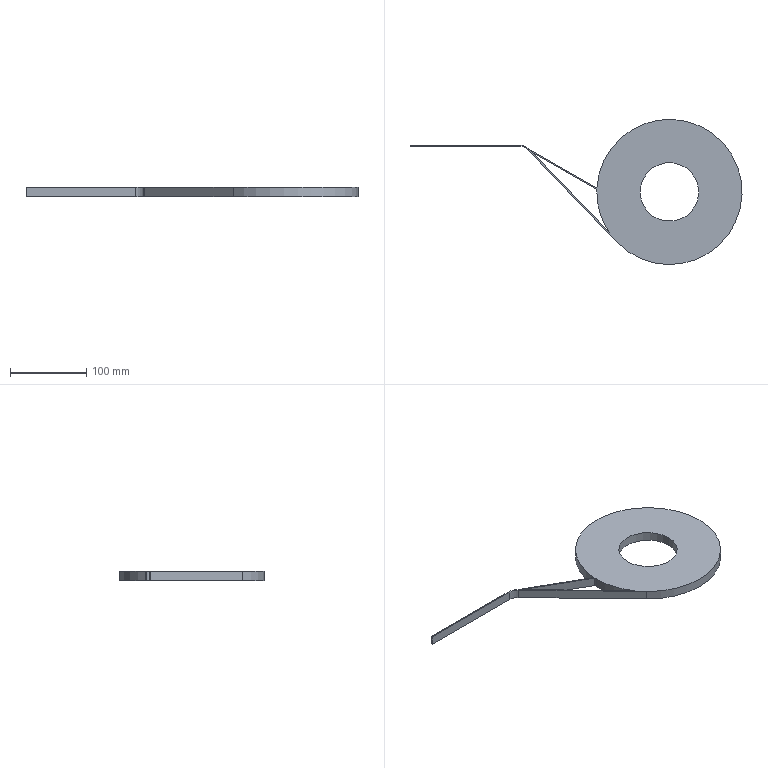Part | STEP file | Mount electronic clip linear-type part | 1 solid | 19 faces | box 434.57 x 190 x 12 mm | volume 291791 mm3 | plane 12 | cylinder 7 | commonest cylinder face diameters 190 x3 76.5 x2 30 x1 32.6 x1
STEP:
#1=CARTESIAN_POINT('',(0.,0.,0.));
#2=DIRECTION('',(0.,0.,1.));
#3=DIRECTION('',(1.,0.,0.));
#4=AXIS2_PLACEMENT_3D('',#1,#2,#3);
#5=CARTESIAN_POINT('',(-95.,0.,6.));
#6=VERTEX_POINT('',#5);
#7=CARTESIAN_POINT('',(-78.379,-53.682,6.));
#8=VERTEX_POINT('',#7);
#9=CARTESIAN_POINT('',(0.,0.,6.));
#10=DIRECTION('',(0.,0.,1.));
#11=DIRECTION('',(1.,0.,0.));
#12=AXIS2_PLACEMENT_3D('',#9,#10,#11);
#13=CIRCLE('',#12,95.);
#14=CARTESIAN_POINT('',(0.,0.,6.));
#15=DIRECTION('',(0.,0.,-1.));
#16=DIRECTION('',(-1.,0.,0.));
#17=AXIS2_PLACEMENT_3D('',#14,#15,#16);
#18=CYLINDRICAL_SURFACE('',#17,95.);
#19=CARTESIAN_POINT('',(9.425,0.));
#20=DIRECTION('',(-1.,0.));
#21=VECTOR('',#20,1.);
#22=LINE('',#19,#21);
#23=(GEOMETRIC_REPRESENTATION_CONTEXT(2)PARAMETRIC_REPRESENTATION_CONTEXT()REPRESENTATION_CONTEXT('',''));
#24=DEFINITIONAL_REPRESENTATION('',(#22),#23);
#25=PCURVE('',#18,#24);
#26=CARTESIAN_POINT('',(0.,0.,6.));
#27=DIRECTION('',(0.,0.,1.));
#28=DIRECTION('',(1.,0.,0.));
#29=AXIS2_PLACEMENT_3D('',#26,#27,#28);
#30=PLANE('',#29);
#31=CARTESIAN_POINT('',(0.,0.));
#32=DIRECTION('',(1.,0.));
#33=AXIS2_PLACEMENT_2D('',#31,#32);
#34=CIRCLE('',#33,95.);
#35=(GEOMETRIC_REPRESENTATION_CONTEXT(2)PARAMETRIC_REPRESENTATION_CONTEXT()REPRESENTATION_CONTEXT('',''));
#36=DEFINITIONAL_REPRESENTATION('',(#34),#35);
#37=PCURVE('',#30,#36);
#38=SURFACE_CURVE('',#13,(#25,#37),.PCURVE_S1.);
#39=EDGE_CURVE('',#6,#8,#38,.T.);
#40=ORIENTED_EDGE('',*,*,#39,.F.);
#41=CARTESIAN_POINT('',(-95.,0.,-6.));
#42=VERTEX_POINT('',#41);
#43=CARTESIAN_POINT('',(-95.,0.,6.));
#44=DIRECTION('',(0.,0.,-1.));
#45=VECTOR('',#44,1.);
#46=LINE('',#43,#45);
#47=CARTESIAN_POINT('',(6.283,0.));
#48=DIRECTION('',(0.,1.));
#49=VECTOR('',#48,1.);
#50=LINE('',#47,#49);
#51=(GEOMETRIC_REPRESENTATION_CONTEXT(2)PARAMETRIC_REPRESENTATION_CONTEXT()REPRESENTATION_CONTEXT('',''));
#52=DEFINITIONAL_REPRESENTATION('',(#50),#51);
#53=PCURVE('',#18,#52);
#54=CARTESIAN_POINT('',(0.,0.,6.));
#55=DIRECTION('',(0.,0.,-1.));
#56=DIRECTION('',(-1.,0.,0.));
#57=AXIS2_PLACEMENT_3D('',#54,#55,#56);
#58=CYLINDRICAL_SURFACE('',#57,95.);
#59=CARTESIAN_POINT('',(0.,0.));
#60=DIRECTION('',(0.,1.));
#61=VECTOR('',#60,1.);
#62=LINE('',#59,#61);
#63=(GEOMETRIC_REPRESENTATION_CONTEXT(2)PARAMETRIC_REPRESENTATION_CONTEXT()REPRESENTATION_CONTEXT('',''));
#64=DEFINITIONAL_REPRESENTATION('',(#62),#63);
#65=PCURVE('',#58,#64);
#66=SURFACE_CURVE('',#46,(#53,#65),.PCURVE_S1.);
#67=EDGE_CURVE('',#6,#42,#66,.T.);
#68=ORIENTED_EDGE('',*,*,#67,.T.);
#69=CARTESIAN_POINT('',(-78.379,-53.682,-6.));
#70=VERTEX_POINT('',#69);
#71=CARTESIAN_POINT('',(0.,0.,-6.));
#72=DIRECTION('',(0.,0.,1.));
#73=DIRECTION('',(1.,0.,0.));
#74=AXIS2_PLACEMENT_3D('',#71,#72,#73);
#75=CIRCLE('',#74,95.);
#76=CARTESIAN_POINT('',(9.425,12.));
#77=DIRECTION('',(-1.,0.));
#78=VECTOR('',#77,1.);
#79=LINE('',#76,#78);
#80=(GEOMETRIC_REPRESENTATION_CONTEXT(2)PARAMETRIC_REPRESENTATION_CONTEXT()REPRESENTATION_CONTEXT('',''));
#81=DEFINITIONAL_REPRESENTATION('',(#79),#80);
#82=PCURVE('',#18,#81);
#83=CARTESIAN_POINT('',(0.,0.,-6.));
#84=DIRECTION('',(0.,0.,1.));
#85=DIRECTION('',(1.,0.,0.));
#86=AXIS2_PLACEMENT_3D('',#83,#84,#85);
#87=PLANE('',#86);
#88=CARTESIAN_POINT('',(0.,0.));
#89=DIRECTION('',(1.,0.));
#90=AXIS2_PLACEMENT_2D('',#88,#89);
#91=CIRCLE('',#90,95.);
#92=(GEOMETRIC_REPRESENTATION_CONTEXT(2)PARAMETRIC_REPRESENTATION_CONTEXT()REPRESENTATION_CONTEXT('',''));
#93=DEFINITIONAL_REPRESENTATION('',(#91),#92);
#94=PCURVE('',#87,#93);
#95=SURFACE_CURVE('',#75,(#82,#94),.PCURVE_S1.);
#96=EDGE_CURVE('',#42,#70,#95,.T.);
#97=ORIENTED_EDGE('',*,*,#96,.T.);
#98=CARTESIAN_POINT('',(-78.379,-53.682,6.));
#99=DIRECTION('',(0.,0.,-1.));
#100=VECTOR('',#99,1.);
#101=LINE('',#98,#100);
#102=CARTESIAN_POINT('',(5.683,0.));
#103=DIRECTION('',(0.,1.));
#104=VECTOR('',#103,1.);
#105=LINE('',#102,#104);
#106=(GEOMETRIC_REPRESENTATION_CONTEXT(2)PARAMETRIC_REPRESENTATION_CONTEXT()REPRESENTATION_CONTEXT('',''));
#107=DEFINITIONAL_REPRESENTATION('',(#105),#106);
#108=PCURVE('',#18,#107);
#109=CARTESIAN_POINT('',(-67.519,-64.968,6.));
#110=DIRECTION('',(-0.7206,-0.6934,0.));
#111=DIRECTION('',(0.6934,-0.7206,0.));
#112=AXIS2_PLACEMENT_3D('',#109,#110,#111);
#113=PLANE('',#112);
#114=CARTESIAN_POINT('',(-15.662,0.));
#115=DIRECTION('',(0.,-1.));
#116=VECTOR('',#115,1.);
#117=LINE('',#114,#116);
#118=(GEOMETRIC_REPRESENTATION_CONTEXT(2)PARAMETRIC_REPRESENTATION_CONTEXT()REPRESENTATION_CONTEXT('',''));
#119=DEFINITIONAL_REPRESENTATION('',(#117),#118);
#120=PCURVE('',#113,#119);
#121=SURFACE_CURVE('',#101,(#108,#120),.PCURVE_S1.);
#122=EDGE_CURVE('',#8,#70,#121,.T.);
#123=ORIENTED_EDGE('',*,*,#122,.F.);
#124=EDGE_LOOP('',(#40,#68,#97,#123));
#125=FACE_BOUND('',#124,.T.);
#126=ADVANCED_FACE('',(#125),#18,.T.);
#127=CARTESIAN_POINT('',(-38.25,0.,6.));
#128=VERTEX_POINT('',#127);
#129=CARTESIAN_POINT('',(-38.25,0.,-6.));
#130=VERTEX_POINT('',#129);
#131=CARTESIAN_POINT('',(-38.25,0.,6.));
#132=DIRECTION('',(0.,0.,-1.));
#133=VECTOR('',#132,1.);
#134=LINE('',#131,#133);
#135=CARTESIAN_POINT('',(0.,0.,6.));
#136=DIRECTION('',(0.,0.,-1.));
#137=DIRECTION('',(-1.,0.,0.));
#138=AXIS2_PLACEMENT_3D('',#135,#136,#137);
#139=CYLINDRICAL_SURFACE('',#138,38.25);
#140=CARTESIAN_POINT('',(6.283,0.));
#141=DIRECTION('',(0.,1.));
#142=VECTOR('',#141,1.);
#143=LINE('',#140,#142);
#144=(GEOMETRIC_REPRESENTATION_CONTEXT(2)PARAMETRIC_REPRESENTATION_CONTEXT()REPRESENTATION_CONTEXT('',''));
#145=DEFINITIONAL_REPRESENTATION('',(#143),#144);
#146=PCURVE('',#139,#145);
#147=CARTESIAN_POINT('',(0.,0.,6.));
#148=DIRECTION('',(0.,0.,-1.));
#149=DIRECTION('',(-1.,0.,0.));
#150=AXIS2_PLACEMENT_3D('',#147,#148,#149);
#151=CYLINDRICAL_SURFACE('',#150,38.25);
#152=CARTESIAN_POINT('',(0.,0.));
#153=DIRECTION('',(0.,1.));
#154=VECTOR('',#153,1.);
#155=LINE('',#152,#154);
#156=(GEOMETRIC_REPRESENTATION_CONTEXT(2)PARAMETRIC_REPRESENTATION_CONTEXT()REPRESENTATION_CONTEXT('',''));
#157=DEFINITIONAL_REPRESENTATION('',(#155),#156);
#158=PCURVE('',#151,#157);
#159=SURFACE_CURVE('',#134,(#146,#158),.PCURVE_S1.);
#160=EDGE_CURVE('',#128,#130,#159,.T.);
#161=ORIENTED_EDGE('',*,*,#160,.T.);
#162=CARTESIAN_POINT('',(38.25,0.,-6.));
#163=VERTEX_POINT('',#162);
#164=CARTESIAN_POINT('',(0.,0.,-6.));
#165=DIRECTION('',(0.,0.,1.));
#166=DIRECTION('',(1.,0.,0.));
#167=AXIS2_PLACEMENT_3D('',#164,#165,#166);
#168=CIRCLE('',#167,38.25);
#169=CARTESIAN_POINT('',(9.425,12.));
#170=DIRECTION('',(-1.,0.));
#171=VECTOR('',#170,1.);
#172=LINE('',#169,#171);
#173=(GEOMETRIC_REPRESENTATION_CONTEXT(2)PARAMETRIC_REPRESENTATION_CONTEXT()REPRESENTATION_CONTEXT('',''));
#174=DEFINITIONAL_REPRESENTATION('',(#172),#173);
#175=PCURVE('',#139,#174);
#176=CARTESIAN_POINT('',(0.,0.));
#177=DIRECTION('',(1.,0.));
#178=AXIS2_PLACEMENT_2D('',#176,#177);
#179=CIRCLE('',#178,38.25);
#180=(GEOMETRIC_REPRESENTATION_CONTEXT(2)PARAMETRIC_REPRESENTATION_CONTEXT()REPRESENTATION_CONTEXT('',''));
#181=DEFINITIONAL_REPRESENTATION('',(#179),#180);
#182=PCURVE('',#87,#181);
#183=SURFACE_CURVE('',#168,(#175,#182),.PCURVE_S1.);
#184=EDGE_CURVE('',#130,#163,#183,.T.);
#185=ORIENTED_EDGE('',*,*,#184,.T.);
#186=CARTESIAN_POINT('',(38.25,0.,6.));
#187=VERTEX_POINT('',#186);
#188=CARTESIAN_POINT('',(38.25,0.,6.));
#189=DIRECTION('',(0.,0.,-1.));
#190=VECTOR('',#189,1.);
#191=LINE('',#188,#190);
#192=CARTESIAN_POINT('',(3.142,0.));
#193=DIRECTION('',(0.,1.));
#194=VECTOR('',#193,1.);
#195=LINE('',#192,#194);
#196=(GEOMETRIC_REPRESENTATION_CONTEXT(2)PARAMETRIC_REPRESENTATION_CONTEXT()REPRESENTATION_CONTEXT('',''));
#197=DEFINITIONAL_REPRESENTATION('',(#195),#196);
#198=PCURVE('',#139,#197);
#199=CARTESIAN_POINT('',(3.142,0.));
#200=DIRECTION('',(0.,1.));
#201=VECTOR('',#200,1.);
#202=LINE('',#199,#201);
#203=(GEOMETRIC_REPRESENTATION_CONTEXT(2)PARAMETRIC_REPRESENTATION_CONTEXT()REPRESENTATION_CONTEXT('',''));
#204=DEFINITIONAL_REPRESENTATION('',(#202),#203);
#205=PCURVE('',#151,#204);
#206=SURFACE_CURVE('',#191,(#198,#205),.PCURVE_S1.);
#207=EDGE_CURVE('',#187,#163,#206,.T.);
#208=ORIENTED_EDGE('',*,*,#207,.F.);
#209=CARTESIAN_POINT('',(0.,0.,6.));
#210=DIRECTION('',(0.,0.,1.));
#211=DIRECTION('',(1.,0.,0.));
#212=AXIS2_PLACEMENT_3D('',#209,#210,#211);
#213=CIRCLE('',#212,38.25);
#214=CARTESIAN_POINT('',(9.425,0.));
#215=DIRECTION('',(-1.,0.));
#216=VECTOR('',#215,1.);
#217=LINE('',#214,#216);
#218=(GEOMETRIC_REPRESENTATION_CONTEXT(2)PARAMETRIC_REPRESENTATION_CONTEXT()REPRESENTATION_CONTEXT('',''));
#219=DEFINITIONAL_REPRESENTATION('',(#217),#218);
#220=PCURVE('',#139,#219);
#221=CARTESIAN_POINT('',(0.,0.));
#222=DIRECTION('',(1.,0.));
#223=AXIS2_PLACEMENT_2D('',#221,#222);
#224=CIRCLE('',#223,38.25);
#225=(GEOMETRIC_REPRESENTATION_CONTEXT(2)PARAMETRIC_REPRESENTATION_CONTEXT()REPRESENTATION_CONTEXT('',''));
#226=DEFINITIONAL_REPRESENTATION('',(#224),#225);
#227=PCURVE('',#30,#226);
#228=SURFACE_CURVE('',#213,(#220,#227),.PCURVE_S1.);
#229=EDGE_CURVE('',#128,#187,#228,.T.);
#230=ORIENTED_EDGE('',*,*,#229,.F.);
#231=EDGE_LOOP('',(#161,#185,#208,#230));
#232=FACE_BOUND('',#231,.F.);
#233=ADVANCED_FACE('',(#232),#139,.F.);
#234=CARTESIAN_POINT('',(-94.855,5.249,6.));
#235=VERTEX_POINT('',#234);
#236=CARTESIAN_POINT('',(-94.855,5.249,-6.));
#237=VERTEX_POINT('',#236);
#238=CARTESIAN_POINT('',(-94.855,5.249,6.));
#239=DIRECTION('',(0.,0.,-1.));
#240=VECTOR('',#239,1.);
#241=LINE('',#238,#240);
#242=CARTESIAN_POINT('',(0.,0.,6.));
#243=DIRECTION('',(0.,0.,-1.));
#244=DIRECTION('',(-1.,0.,0.));
#245=AXIS2_PLACEMENT_3D('',#242,#243,#244);
#246=CYLINDRICAL_SURFACE('',#245,95.);
#247=CARTESIAN_POINT('',(0.05528,0.));
#248=DIRECTION('',(0.,1.));
#249=VECTOR('',#248,1.);
#250=LINE('',#247,#249);
#251=(GEOMETRIC_REPRESENTATION_CONTEXT(2)PARAMETRIC_REPRESENTATION_CONTEXT()REPRESENTATION_CONTEXT('',''));
#252=DEFINITIONAL_REPRESENTATION('',(#250),#251);
#253=PCURVE('',#246,#252);
#254=CARTESIAN_POINT('',(-21.084,-36.901,195.166));
#255=DIRECTION('',(-0.4961,-0.8683,0.));
#256=DIRECTION('',(0.8683,-0.4961,0.));
#257=AXIS2_PLACEMENT_3D('',#254,#255,#256);
#258=PLANE('',#257);
#259=CARTESIAN_POINT('',(-84.963,-189.166));
#260=DIRECTION('',(0.,-1.));
#261=VECTOR('',#260,1.);
#262=LINE('',#259,#261);
#263=(GEOMETRIC_REPRESENTATION_CONTEXT(2)PARAMETRIC_REPRESENTATION_CONTEXT()REPRESENTATION_CONTEXT('',''));
#264=DEFINITIONAL_REPRESENTATION('',(#262),#263);
#265=PCURVE('',#258,#264);
#266=SURFACE_CURVE('',#241,(#253,#265),.PCURVE_S1.);
#267=EDGE_CURVE('',#235,#237,#266,.T.);
#268=ORIENTED_EDGE('',*,*,#267,.F.);
#269=CARTESIAN_POINT('',(-68.456,-65.87,6.));
#270=VERTEX_POINT('',#269);
#271=CARTESIAN_POINT('',(0.,0.,6.));
#272=DIRECTION('',(0.,0.,1.));
#273=DIRECTION('',(1.,0.,0.));
#274=AXIS2_PLACEMENT_3D('',#271,#272,#273);
#275=CIRCLE('',#274,95.);
#276=CARTESIAN_POINT('',(9.425,0.));
#277=DIRECTION('',(-1.,0.));
#278=VECTOR('',#277,1.);
#279=LINE('',#276,#278);
#280=(GEOMETRIC_REPRESENTATION_CONTEXT(2)PARAMETRIC_REPRESENTATION_CONTEXT()REPRESENTATION_CONTEXT('',''));
#281=DEFINITIONAL_REPRESENTATION('',(#279),#280);
#282=PCURVE('',#246,#281);
#283=CARTESIAN_POINT('',(0.,0.));
#284=DIRECTION('',(1.,0.));
#285=AXIS2_PLACEMENT_2D('',#283,#284);
#286=CIRCLE('',#285,95.);
#287=(GEOMETRIC_REPRESENTATION_CONTEXT(2)PARAMETRIC_REPRESENTATION_CONTEXT()REPRESENTATION_CONTEXT('',''));
#288=DEFINITIONAL_REPRESENTATION('',(#286),#287);
#289=PCURVE('',#30,#288);
#290=SURFACE_CURVE('',#275,(#282,#289),.PCURVE_S1.);
#291=EDGE_CURVE('',#270,#235,#290,.T.);
#292=ORIENTED_EDGE('',*,*,#291,.F.);
#293=CARTESIAN_POINT('',(-68.456,-65.87,-6.));
#294=VERTEX_POINT('',#293);
#295=CARTESIAN_POINT('',(-68.456,-65.87,6.));
#296=DIRECTION('',(0.,0.,-1.));
#297=VECTOR('',#296,1.);
#298=LINE('',#295,#297);
#299=CARTESIAN_POINT('',(5.517,0.));
#300=DIRECTION('',(0.,1.));
#301=VECTOR('',#300,1.);
#302=LINE('',#299,#301);
#303=(GEOMETRIC_REPRESENTATION_CONTEXT(2)PARAMETRIC_REPRESENTATION_CONTEXT()REPRESENTATION_CONTEXT('',''));
#304=DEFINITIONAL_REPRESENTATION('',(#302),#303);
#305=PCURVE('',#246,#304);
#306=CARTESIAN_POINT('',(-68.456,-65.87,6.));
#307=DIRECTION('',(-0.7206,-0.6934,0.));
#308=DIRECTION('',(0.6934,-0.7206,0.));
#309=AXIS2_PLACEMENT_3D('',#306,#307,#308);
#310=PLANE('',#309);
#311=CARTESIAN_POINT('',(0.,0.));
#312=DIRECTION('',(0.,-1.));
#313=VECTOR('',#312,1.);
#314=LINE('',#311,#313);
#315=(GEOMETRIC_REPRESENTATION_CONTEXT(2)PARAMETRIC_REPRESENTATION_CONTEXT()REPRESENTATION_CONTEXT('',''));
#316=DEFINITIONAL_REPRESENTATION('',(#314),#315);
#317=PCURVE('',#310,#316);
#318=SURFACE_CURVE('',#298,(#305,#317),.PCURVE_S1.);
#319=EDGE_CURVE('',#270,#294,#318,.T.);
#320=ORIENTED_EDGE('',*,*,#319,.T.);
#321=CARTESIAN_POINT('',(0.,0.,-6.));
#322=DIRECTION('',(0.,0.,1.));
#323=DIRECTION('',(1.,0.,0.));
#324=AXIS2_PLACEMENT_3D('',#321,#322,#323);
#325=CIRCLE('',#324,95.);
#326=CARTESIAN_POINT('',(9.425,12.));
#327=DIRECTION('',(-1.,0.));
#328=VECTOR('',#327,1.);
#329=LINE('',#326,#328);
#330=(GEOMETRIC_REPRESENTATION_CONTEXT(2)PARAMETRIC_REPRESENTATION_CONTEXT()REPRESENTATION_CONTEXT('',''));
#331=DEFINITIONAL_REPRESENTATION('',(#329),#330);
#332=PCURVE('',#246,#331);
#333=CARTESIAN_POINT('',(0.,0.));
#334=DIRECTION('',(1.,0.));
#335=AXIS2_PLACEMENT_2D('',#333,#334);
#336=CIRCLE('',#335,95.);
#337=(GEOMETRIC_REPRESENTATION_CONTEXT(2)PARAMETRIC_REPRESENTATION_CONTEXT()REPRESENTATION_CONTEXT('',''));
#338=DEFINITIONAL_REPRESENTATION('',(#336),#337);
#339=PCURVE('',#87,#338);
#340=SURFACE_CURVE('',#325,(#332,#339),.PCURVE_S1.);
#341=EDGE_CURVE('',#294,#237,#340,.T.);
#342=ORIENTED_EDGE('',*,*,#341,.T.);
#343=EDGE_LOOP('',(#268,#292,#320,#342));
#344=FACE_BOUND('',#343,.T.);
#345=ADVANCED_FACE('',(#344),#246,.T.);
#346=CARTESIAN_POINT('',(-184.88,55.125,-6.));
#347=VERTEX_POINT('',#346);
#348=CARTESIAN_POINT('',(-185.144,55.4,-6.));
#349=VERTEX_POINT('',#348);
#350=CARTESIAN_POINT('',(-68.456,-65.87,-6.));
#351=DIRECTION('',(-0.6934,0.7206,0.));
#352=VECTOR('',#351,1.);
#353=LINE('',#350,#352);
#354=CARTESIAN_POINT('',(-68.456,-65.87,6.));
#355=DIRECTION('',(-0.7206,-0.6934,0.));
#356=DIRECTION('',(0.6934,-0.7206,0.));
#357=AXIS2_PLACEMENT_3D('',#354,#355,#356);
#358=PLANE('',#357);
#359=CARTESIAN_POINT('',(0.,-12.));
#360=DIRECTION('',(-1.,0.));
#361=VECTOR('',#360,1.);
#362=LINE('',#359,#361);
#363=(GEOMETRIC_REPRESENTATION_CONTEXT(2)PARAMETRIC_REPRESENTATION_CONTEXT()REPRESENTATION_CONTEXT('',''));
#364=DEFINITIONAL_REPRESENTATION('',(#362),#363);
#365=PCURVE('',#358,#364);
#366=CARTESIAN_POINT('',(-68.456,-65.87));
#367=DIRECTION('',(-0.6934,0.7206));
#368=VECTOR('',#367,1.);
#369=LINE('',#366,#368);
#370=(GEOMETRIC_REPRESENTATION_CONTEXT(2)PARAMETRIC_REPRESENTATION_CONTEXT()REPRESENTATION_CONTEXT('',''));
#371=DEFINITIONAL_REPRESENTATION('',(#369),#370);
#372=PCURVE('',#87,#371);
#373=SURFACE_CURVE('',#353,(#365,#372),.PCURVE_S1.);
#374=EDGE_CURVE('',#347,#349,#373,.T.);
#375=ORIENTED_EDGE('',*,*,#374,.F.);
#376=CARTESIAN_POINT('',(-184.88,55.125,6.));
#377=VERTEX_POINT('',#376);
#378=CARTESIAN_POINT('',(-184.88,55.125,6.));
#379=DIRECTION('',(0.,0.,1.));
#380=VECTOR('',#379,1.);
#381=LINE('',#378,#380);
#382=CARTESIAN_POINT('',(-167.912,0.));
#383=DIRECTION('',(0.,1.));
#384=VECTOR('',#383,1.);
#385=LINE('',#382,#384);
#386=(GEOMETRIC_REPRESENTATION_CONTEXT(2)PARAMETRIC_REPRESENTATION_CONTEXT()REPRESENTATION_CONTEXT('',''));
#387=DEFINITIONAL_REPRESENTATION('',(#385),#386);
#388=PCURVE('',#358,#387);
#389=CARTESIAN_POINT('',(-184.207,56.302,195.166));
#390=DIRECTION('',(0.8683,-0.4961,0.));
#391=DIRECTION('',(0.4961,0.8683,0.));
#392=AXIS2_PLACEMENT_3D('',#389,#390,#391);
#393=PLANE('',#392);
#394=CARTESIAN_POINT('',(-1.355,-189.166));
#395=DIRECTION('',(0.,1.));
#396=VECTOR('',#395,1.);
#397=LINE('',#394,#396);
#398=(GEOMETRIC_REPRESENTATION_CONTEXT(2)PARAMETRIC_REPRESENTATION_CONTEXT()REPRESENTATION_CONTEXT('',''));
#399=DEFINITIONAL_REPRESENTATION('',(#397),#398);
#400=PCURVE('',#393,#399);
#401=SURFACE_CURVE('',#381,(#388,#400),.PCURVE_S1.);
#402=EDGE_CURVE('',#347,#377,#401,.T.);
#403=ORIENTED_EDGE('',*,*,#402,.T.);
#404=CARTESIAN_POINT('',(-185.144,55.4,6.));
#405=VERTEX_POINT('',#404);
#406=CARTESIAN_POINT('',(-68.456,-65.87,6.));
#407=DIRECTION('',(-0.6934,0.7206,0.));
#408=VECTOR('',#407,1.);
#409=LINE('',#406,#408);
#410=CARTESIAN_POINT('',(0.,0.));
#411=DIRECTION('',(-1.,0.));
#412=VECTOR('',#411,1.);
#413=LINE('',#410,#412);
#414=(GEOMETRIC_REPRESENTATION_CONTEXT(2)PARAMETRIC_REPRESENTATION_CONTEXT()REPRESENTATION_CONTEXT('',''));
#415=DEFINITIONAL_REPRESENTATION('',(#413),#414);
#416=PCURVE('',#358,#415);
#417=CARTESIAN_POINT('',(-68.456,-65.87));
#418=DIRECTION('',(-0.6934,0.7206));
#419=VECTOR('',#418,1.);
#420=LINE('',#417,#419);
#421=(GEOMETRIC_REPRESENTATION_CONTEXT(2)PARAMETRIC_REPRESENTATION_CONTEXT()REPRESENTATION_CONTEXT('',''));
#422=DEFINITIONAL_REPRESENTATION('',(#420),#421);
#423=PCURVE('',#30,#422);
#424=SURFACE_CURVE('',#409,(#416,#423),.PCURVE_S1.);
#425=EDGE_CURVE('',#377,#405,#424,.T.);
#426=ORIENTED_EDGE('',*,*,#425,.T.);
#427=CARTESIAN_POINT('',(-185.144,55.4,6.));
#428=DIRECTION('',(0.,0.,-1.));
#429=VECTOR('',#428,1.);
#430=LINE('',#427,#429);
#431=CARTESIAN_POINT('',(-168.293,0.));
#432=DIRECTION('',(0.,-1.));
#433=VECTOR('',#432,1.);
#434=LINE('',#431,#433);
#435=(GEOMETRIC_REPRESENTATION_CONTEXT(2)PARAMETRIC_REPRESENTATION_CONTEXT()REPRESENTATION_CONTEXT('',''));
#436=DEFINITIONAL_REPRESENTATION('',(#434),#435);
#437=PCURVE('',#358,#436);
#438=CARTESIAN_POINT('',(-195.953,45.,6.));
#439=DIRECTION('',(0.,0.,-1.));
#440=DIRECTION('',(-1.,0.,0.));
#441=AXIS2_PLACEMENT_3D('',#438,#439,#440);
#442=CYLINDRICAL_SURFACE('',#441,15.);
#443=CARTESIAN_POINT('',(2.375,0.));
#444=DIRECTION('',(0.,1.));
#445=VECTOR('',#444,1.);
#446=LINE('',#443,#445);
#447=(GEOMETRIC_REPRESENTATION_CONTEXT(2)PARAMETRIC_REPRESENTATION_CONTEXT()REPRESENTATION_CONTEXT('',''));
#448=DEFINITIONAL_REPRESENTATION('',(#446),#447);
#449=PCURVE('',#442,#448);
#450=SURFACE_CURVE('',#430,(#437,#449),.PCURVE_S1.);
#451=EDGE_CURVE('',#405,#349,#450,.T.);
#452=ORIENTED_EDGE('',*,*,#451,.T.);
#453=EDGE_LOOP('',(#375,#403,#426,#452));
#454=FACE_BOUND('',#453,.T.);
#455=ADVANCED_FACE('',(#454),#358,.T.);
#456=CARTESIAN_POINT('',(-180.515,52.465,6.));
#457=VERTEX_POINT('',#456);
#458=CARTESIAN_POINT('',(-67.519,-64.968,6.));
#459=DIRECTION('',(-0.6934,0.7206,0.));
#460=VECTOR('',#459,1.);
#461=LINE('',#458,#460);
#462=CARTESIAN_POINT('',(-67.519,-64.968));
#463=DIRECTION('',(-0.6934,0.7206));
#464=VECTOR('',#463,1.);
#465=LINE('',#462,#464);
#466=(GEOMETRIC_REPRESENTATION_CONTEXT(2)PARAMETRIC_REPRESENTATION_CONTEXT()REPRESENTATION_CONTEXT('',''));
#467=DEFINITIONAL_REPRESENTATION('',(#465),#466);
#468=PCURVE('',#30,#467);
#469=CARTESIAN_POINT('',(0.,0.));
#470=DIRECTION('',(-1.,0.));
#471=VECTOR('',#470,1.);
#472=LINE('',#469,#471);
#473=(GEOMETRIC_REPRESENTATION_CONTEXT(2)PARAMETRIC_REPRESENTATION_CONTEXT()REPRESENTATION_CONTEXT('',''));
#474=DEFINITIONAL_REPRESENTATION('',(#472),#473);
#475=PCURVE('',#113,#474);
#476=SURFACE_CURVE('',#461,(#468,#475),.PCURVE_S1.);
#477=EDGE_CURVE('',#8,#457,#476,.T.);
#478=ORIENTED_EDGE('',*,*,#477,.T.);
#479=CARTESIAN_POINT('',(-94.933,3.566,6.));
#480=VERTEX_POINT('',#479);
#481=CARTESIAN_POINT('',(-21.828,-38.204,6.));
#482=DIRECTION('',(-0.8683,0.4961,0.));
#483=VECTOR('',#482,1.);
#484=LINE('',#481,#483);
#485=CARTESIAN_POINT('',(-21.828,-38.204));
#486=DIRECTION('',(-0.8683,0.4961));
#487=VECTOR('',#486,1.);
#488=LINE('',#485,#487);
#489=(GEOMETRIC_REPRESENTATION_CONTEXT(2)PARAMETRIC_REPRESENTATION_CONTEXT()REPRESENTATION_CONTEXT('',''));
#490=DEFINITIONAL_REPRESENTATION('',(#488),#489);
#491=PCURVE('',#30,#490);
#492=CARTESIAN_POINT('',(-21.828,-38.204,195.166));
#493=DIRECTION('',(-0.4961,-0.8683,0.));
#494=DIRECTION('',(0.8683,-0.4961,0.));
#495=AXIS2_PLACEMENT_3D('',#492,#493,#494);
#496=PLANE('',#495);
#497=CARTESIAN_POINT('',(0.,-189.166));
#498=DIRECTION('',(-1.,0.));
#499=VECTOR('',#498,1.);
#500=LINE('',#497,#499);
#501=(GEOMETRIC_REPRESENTATION_CONTEXT(2)PARAMETRIC_REPRESENTATION_CONTEXT()REPRESENTATION_CONTEXT('',''));
#502=DEFINITIONAL_REPRESENTATION('',(#500),#501);
#503=PCURVE('',#496,#502);
#504=SURFACE_CURVE('',#484,(#491,#503),.PCURVE_S1.);
#505=EDGE_CURVE('',#480,#457,#504,.T.);
#506=ORIENTED_EDGE('',*,*,#505,.F.);
#507=CARTESIAN_POINT('',(0.,0.,6.));
#508=DIRECTION('',(0.,0.,1.));
#509=DIRECTION('',(1.,0.,0.));
#510=AXIS2_PLACEMENT_3D('',#507,#508,#509);
#511=CIRCLE('',#510,95.);
#512=CARTESIAN_POINT('',(0.,0.));
#513=DIRECTION('',(1.,0.));
#514=AXIS2_PLACEMENT_2D('',#512,#513);
#515=CIRCLE('',#514,95.);
#516=(GEOMETRIC_REPRESENTATION_CONTEXT(2)PARAMETRIC_REPRESENTATION_CONTEXT()REPRESENTATION_CONTEXT('',''));
#517=DEFINITIONAL_REPRESENTATION('',(#515),#516);
#518=PCURVE('',#30,#517);
#519=CARTESIAN_POINT('',(3.142,0.));
#520=DIRECTION('',(-1.,0.));
#521=VECTOR('',#520,1.);
#522=LINE('',#519,#521);
#523=(GEOMETRIC_REPRESENTATION_CONTEXT(2)PARAMETRIC_REPRESENTATION_CONTEXT()REPRESENTATION_CONTEXT('',''));
#524=DEFINITIONAL_REPRESENTATION('',(#522),#523);
#525=PCURVE('',#58,#524);
#526=SURFACE_CURVE('',#511,(#518,#525),.PCURVE_S1.);
#527=EDGE_CURVE('',#480,#6,#526,.T.);
#528=ORIENTED_EDGE('',*,*,#527,.T.);
#529=ORIENTED_EDGE('',*,*,#39,.T.);
#530=EDGE_LOOP('',(#478,#506,#528,#529));
#531=FACE_BOUND('',#530,.T.);
#532=CARTESIAN_POINT('',(-184.522,54.754,6.));
#533=VERTEX_POINT('',#532);
#534=CARTESIAN_POINT('',(-184.952,54.999,6.));
#535=VERTEX_POINT('',#534);
#536=CARTESIAN_POINT('',(-21.828,-38.204,6.));
#537=DIRECTION('',(-0.8683,0.4961,0.));
#538=VECTOR('',#537,1.);
#539=LINE('',#536,#538);
#540=CARTESIAN_POINT('',(-21.828,-38.204));
#541=DIRECTION('',(-0.8683,0.4961));
#542=VECTOR('',#541,1.);
#543=LINE('',#540,#542);
#544=(GEOMETRIC_REPRESENTATION_CONTEXT(2)PARAMETRIC_REPRESENTATION_CONTEXT()REPRESENTATION_CONTEXT('',''));
#545=DEFINITIONAL_REPRESENTATION('',(#543),#544);
#546=PCURVE('',#30,#545);
#547=CARTESIAN_POINT('',(-21.828,-38.204,195.166));
#548=DIRECTION('',(-0.4961,-0.8683,0.));
#549=DIRECTION('',(0.8683,-0.4961,0.));
#550=AXIS2_PLACEMENT_3D('',#547,#548,#549);
#551=PLANE('',#550);
#552=CARTESIAN_POINT('',(0.,-189.166));
#553=DIRECTION('',(-1.,0.));
#554=VECTOR('',#553,1.);
#555=LINE('',#552,#554);
#556=(GEOMETRIC_REPRESENTATION_CONTEXT(2)PARAMETRIC_REPRESENTATION_CONTEXT()REPRESENTATION_CONTEXT('',''));
#557=DEFINITIONAL_REPRESENTATION('',(#555),#556);
#558=PCURVE('',#551,#557);
#559=SURFACE_CURVE('',#539,(#546,#558),.PCURVE_S1.);
#560=EDGE_CURVE('',#533,#535,#559,.T.);
#561=ORIENTED_EDGE('',*,*,#560,.F.);
#562=CARTESIAN_POINT('',(-68.456,-65.87,6.));
#563=DIRECTION('',(-0.6934,0.7206,0.));
#564=VECTOR('',#563,1.);
#565=LINE('',#562,#564);
#566=CARTESIAN_POINT('',(-68.456,-65.87));
#567=DIRECTION('',(-0.6934,0.7206));
#568=VECTOR('',#567,1.);
#569=LINE('',#566,#568);
#570=(GEOMETRIC_REPRESENTATION_CONTEXT(2)PARAMETRIC_REPRESENTATION_CONTEXT()REPRESENTATION_CONTEXT('',''));
#571=DEFINITIONAL_REPRESENTATION('',(#569),#570);
#572=PCURVE('',#30,#571);
#573=CARTESIAN_POINT('',(0.,0.));
#574=DIRECTION('',(-1.,0.));
#575=VECTOR('',#574,1.);
#576=LINE('',#573,#575);
#577=(GEOMETRIC_REPRESENTATION_CONTEXT(2)PARAMETRIC_REPRESENTATION_CONTEXT()REPRESENTATION_CONTEXT('',''));
#578=DEFINITIONAL_REPRESENTATION('',(#576),#577);
#579=PCURVE('',#310,#578);
#580=SURFACE_CURVE('',#565,(#572,#579),.PCURVE_S1.);
#581=EDGE_CURVE('',#270,#533,#580,.T.);
#582=ORIENTED_EDGE('',*,*,#581,.F.);
#583=ORIENTED_EDGE('',*,*,#291,.T.);
#584=CARTESIAN_POINT('',(-184.207,56.302,6.));
#585=VERTEX_POINT('',#584);
#586=CARTESIAN_POINT('',(-21.084,-36.901,6.));
#587=DIRECTION('',(-0.8683,0.4961,0.));
#588=VECTOR('',#587,1.);
#589=LINE('',#586,#588);
#590=CARTESIAN_POINT('',(-21.084,-36.901));
#591=DIRECTION('',(-0.8683,0.4961));
#592=VECTOR('',#591,1.);
#593=LINE('',#590,#592);
#594=(GEOMETRIC_REPRESENTATION_CONTEXT(2)PARAMETRIC_REPRESENTATION_CONTEXT()REPRESENTATION_CONTEXT('',''));
#595=DEFINITIONAL_REPRESENTATION('',(#593),#594);
#596=PCURVE('',#30,#595);
#597=CARTESIAN_POINT('',(0.,-189.166));
#598=DIRECTION('',(-1.,0.));
#599=VECTOR('',#598,1.);
#600=LINE('',#597,#599);
#601=(GEOMETRIC_REPRESENTATION_CONTEXT(2)PARAMETRIC_REPRESENTATION_CONTEXT()REPRESENTATION_CONTEXT('',''));
#602=DEFINITIONAL_REPRESENTATION('',(#600),#601);
#603=PCURVE('',#258,#602);
#604=SURFACE_CURVE('',#589,(#596,#603),.PCURVE_S1.);
#605=EDGE_CURVE('',#235,#585,#604,.T.);
#606=ORIENTED_EDGE('',*,*,#605,.T.);
#607=CARTESIAN_POINT('',(-195.953,61.3,6.));
#608=VERTEX_POINT('',#607);
#609=CARTESIAN_POINT('',(-195.953,45.,6.));
#610=DIRECTION('',(0.,0.,1.));
#611=DIRECTION('',(-1.,0.,0.));
#612=AXIS2_PLACEMENT_3D('',#609,#610,#611);
#613=CIRCLE('',#612,16.3);
#614=CARTESIAN_POINT('',(-195.953,45.));
#615=DIRECTION('',(-1.,0.));
#616=AXIS2_PLACEMENT_2D('',#614,#615);
#617=CIRCLE('',#616,16.3);
#618=(GEOMETRIC_REPRESENTATION_CONTEXT(2)PARAMETRIC_REPRESENTATION_CONTEXT()REPRESENTATION_CONTEXT('',''));
#619=DEFINITIONAL_REPRESENTATION('',(#617),#618);
#620=PCURVE('',#30,#619);
#621=CARTESIAN_POINT('',(-195.953,45.,6.));
#622=DIRECTION('',(0.,0.,-1.));
#623=DIRECTION('',(-1.,0.,0.));
#624=AXIS2_PLACEMENT_3D('',#621,#622,#623);
#625=CYLINDRICAL_SURFACE('',#624,16.3);
#626=CARTESIAN_POINT('',(6.283,0.));
#627=DIRECTION('',(-1.,0.));
#628=VECTOR('',#627,1.);
#629=LINE('',#626,#628);
#630=(GEOMETRIC_REPRESENTATION_CONTEXT(2)PARAMETRIC_REPRESENTATION_CONTEXT()REPRESENTATION_CONTEXT('',''));
#631=DEFINITIONAL_REPRESENTATION('',(#629),#630);
#632=PCURVE('',#625,#631);
#633=SURFACE_CURVE('',#613,(#620,#632),.PCURVE_S1.);
#634=EDGE_CURVE('',#585,#608,#633,.T.);
#635=ORIENTED_EDGE('',*,*,#634,.T.);
#636=CARTESIAN_POINT('',(-339.57,61.3,6.));
#637=VERTEX_POINT('',#636);
#638=CARTESIAN_POINT('',(-195.953,61.3,6.));
#639=DIRECTION('',(-1.,0.,0.));
#640=VECTOR('',#639,1.);
#641=LINE('',#638,#640);
#642=CARTESIAN_POINT('',(-195.953,61.3));
#643=DIRECTION('',(-1.,0.));
#644=VECTOR('',#643,1.);
#645=LINE('',#642,#644);
#646=(GEOMETRIC_REPRESENTATION_CONTEXT(2)PARAMETRIC_REPRESENTATION_CONTEXT()REPRESENTATION_CONTEXT('',''));
#647=DEFINITIONAL_REPRESENTATION('',(#645),#646);
#648=PCURVE('',#30,#647);
#649=CARTESIAN_POINT('',(-195.953,61.3,6.));
#650=DIRECTION('',(0.,-1.,0.));
#651=DIRECTION('',(1.,0.,0.));
#652=AXIS2_PLACEMENT_3D('',#649,#650,#651);
#653=PLANE('',#652);
#654=CARTESIAN_POINT('',(0.,0.));
#655=DIRECTION('',(-1.,0.));
#656=VECTOR('',#655,1.);
#657=LINE('',#654,#656);
#658=(GEOMETRIC_REPRESENTATION_CONTEXT(2)PARAMETRIC_REPRESENTATION_CONTEXT()REPRESENTATION_CONTEXT('',''));
#659=DEFINITIONAL_REPRESENTATION('',(#657),#658);
#660=PCURVE('',#653,#659);
#661=SURFACE_CURVE('',#641,(#648,#660),.PCURVE_S1.);
#662=EDGE_CURVE('',#608,#637,#661,.T.);
#663=ORIENTED_EDGE('',*,*,#662,.T.);
#664=CARTESIAN_POINT('',(-339.57,60.,6.));
#665=VERTEX_POINT('',#664);
#666=CARTESIAN_POINT('',(-339.57,61.3,6.));
#667=DIRECTION('',(0.,-1.,0.));
#668=VECTOR('',#667,1.);
#669=LINE('',#666,#668);
#670=CARTESIAN_POINT('',(-339.57,61.3));
#671=DIRECTION('',(0.,-1.));
#672=VECTOR('',#671,1.);
#673=LINE('',#670,#672);
#674=(GEOMETRIC_REPRESENTATION_CONTEXT(2)PARAMETRIC_REPRESENTATION_CONTEXT()REPRESENTATION_CONTEXT('',''));
#675=DEFINITIONAL_REPRESENTATION('',(#673),#674);
#676=PCURVE('',#30,#675);
#677=CARTESIAN_POINT('',(-339.57,61.3,6.));
#678=DIRECTION('',(1.,0.,0.));
#679=DIRECTION('',(0.,0.,-1.));
#680=AXIS2_PLACEMENT_3D('',#677,#678,#679);
#681=PLANE('',#680);
#682=CARTESIAN_POINT('',(0.,0.));
#683=DIRECTION('',(0.,-1.));
#684=VECTOR('',#683,1.);
#685=LINE('',#682,#684);
#686=(GEOMETRIC_REPRESENTATION_CONTEXT(2)PARAMETRIC_REPRESENTATION_CONTEXT()REPRESENTATION_CONTEXT('',''));
#687=DEFINITIONAL_REPRESENTATION('',(#685),#686);
#688=PCURVE('',#681,#687);
#689=SURFACE_CURVE('',#669,(#676,#688),.PCURVE_S1.);
#690=EDGE_CURVE('',#637,#665,#689,.T.);
#691=ORIENTED_EDGE('',*,*,#690,.T.);
#692=CARTESIAN_POINT('',(-195.953,60.,6.));
#693=VERTEX_POINT('',#692);
#694=CARTESIAN_POINT('',(-195.953,60.,6.));
#695=DIRECTION('',(-1.,0.,0.));
#696=VECTOR('',#695,1.);
#697=LINE('',#694,#696);
#698=CARTESIAN_POINT('',(-195.953,60.));
#699=DIRECTION('',(-1.,0.));
#700=VECTOR('',#699,1.);
#701=LINE('',#698,#700);
#702=(GEOMETRIC_REPRESENTATION_CONTEXT(2)PARAMETRIC_REPRESENTATION_CONTEXT()REPRESENTATION_CONTEXT('',''));
#703=DEFINITIONAL_REPRESENTATION('',(#701),#702);
#704=PCURVE('',#30,#703);
#705=CARTESIAN_POINT('',(-195.953,60.,6.));
#706=DIRECTION('',(0.,-1.,0.));
#707=DIRECTION('',(1.,0.,0.));
#708=AXIS2_PLACEMENT_3D('',#705,#706,#707);
#709=PLANE('',#708);
#710=CARTESIAN_POINT('',(0.,0.));
#711=DIRECTION('',(-1.,0.));
#712=VECTOR('',#711,1.);
#713=LINE('',#710,#712);
#714=(GEOMETRIC_REPRESENTATION_CONTEXT(2)PARAMETRIC_REPRESENTATION_CONTEXT()REPRESENTATION_CONTEXT('',''));
#715=DEFINITIONAL_REPRESENTATION('',(#713),#714);
#716=PCURVE('',#709,#715);
#717=SURFACE_CURVE('',#697,(#704,#716),.PCURVE_S1.);
#718=EDGE_CURVE('',#693,#665,#717,.T.);
#719=ORIENTED_EDGE('',*,*,#718,.F.);
#720=CARTESIAN_POINT('',(-195.953,45.,6.));
#721=DIRECTION('',(0.,0.,1.));
#722=DIRECTION('',(1.,0.,0.));
#723=AXIS2_PLACEMENT_3D('',#720,#721,#722);
#724=CIRCLE('',#723,15.);
#725=CARTESIAN_POINT('',(-195.953,45.));
#726=DIRECTION('',(1.,0.));
#727=AXIS2_PLACEMENT_2D('',#725,#726);
#728=CIRCLE('',#727,15.);
#729=(GEOMETRIC_REPRESENTATION_CONTEXT(2)PARAMETRIC_REPRESENTATION_CONTEXT()REPRESENTATION_CONTEXT('',''));
#730=DEFINITIONAL_REPRESENTATION('',(#728),#729);
#731=PCURVE('',#30,#730);
#732=CARTESIAN_POINT('',(3.142,0.));
#733=DIRECTION('',(-1.,0.));
#734=VECTOR('',#733,1.);
#735=LINE('',#732,#734);
#736=(GEOMETRIC_REPRESENTATION_CONTEXT(2)PARAMETRIC_REPRESENTATION_CONTEXT()REPRESENTATION_CONTEXT('',''));
#737=DEFINITIONAL_REPRESENTATION('',(#735),#736);
#738=PCURVE('',#442,#737);
#739=SURFACE_CURVE('',#724,(#731,#738),.PCURVE_S1.);
#740=EDGE_CURVE('',#405,#693,#739,.T.);
#741=ORIENTED_EDGE('',*,*,#740,.F.);
#742=ORIENTED_EDGE('',*,*,#425,.F.);
#743=CARTESIAN_POINT('',(-184.207,56.302,6.));
#744=DIRECTION('',(-0.4961,-0.8683,0.));
#745=VECTOR('',#744,1.);
#746=LINE('',#743,#745);
#747=CARTESIAN_POINT('',(-184.207,56.302));
#748=DIRECTION('',(-0.4961,-0.8683));
#749=VECTOR('',#748,1.);
#750=LINE('',#747,#749);
#751=(GEOMETRIC_REPRESENTATION_CONTEXT(2)PARAMETRIC_REPRESENTATION_CONTEXT()REPRESENTATION_CONTEXT('',''));
#752=DEFINITIONAL_REPRESENTATION('',(#750),#751);
#753=PCURVE('',#30,#752);
#754=CARTESIAN_POINT('',(0.,-189.166));
#755=DIRECTION('',(-1.,0.));
#756=VECTOR('',#755,1.);
#757=LINE('',#754,#756);
#758=(GEOMETRIC_REPRESENTATION_CONTEXT(2)PARAMETRIC_REPRESENTATION_CONTEXT()REPRESENTATION_CONTEXT('',''));
#759=DEFINITIONAL_REPRESENTATION('',(#757),#758);
#760=PCURVE('',#393,#759);
#761=SURFACE_CURVE('',#746,(#753,#760),.PCURVE_S1.);
#762=EDGE_CURVE('',#377,#535,#761,.T.);
#763=ORIENTED_EDGE('',*,*,#762,.T.);
#764=EDGE_LOOP('',(#561,#582,#583,#606,#635,#663,#691,#719,#741,#742,#763));
#765=FACE_BOUND('',#764,.T.);
#766=ORIENTED_EDGE('',*,*,#229,.F.);
#767=CARTESIAN_POINT('',(0.,0.,6.));
#768=DIRECTION('',(0.,0.,1.));
#769=DIRECTION('',(1.,0.,0.));
#770=AXIS2_PLACEMENT_3D('',#767,#768,#769);
#771=CIRCLE('',#770,38.25);
#772=CARTESIAN_POINT('',(0.,0.));
#773=DIRECTION('',(1.,0.));
#774=AXIS2_PLACEMENT_2D('',#772,#773);
#775=CIRCLE('',#774,38.25);
#776=(GEOMETRIC_REPRESENTATION_CONTEXT(2)PARAMETRIC_REPRESENTATION_CONTEXT()REPRESENTATION_CONTEXT('',''));
#777=DEFINITIONAL_REPRESENTATION('',(#775),#776);
#778=PCURVE('',#30,#777);
#779=CARTESIAN_POINT('',(3.142,0.));
#780=DIRECTION('',(-1.,0.));
#781=VECTOR('',#780,1.);
#782=LINE('',#779,#781);
#783=(GEOMETRIC_REPRESENTATION_CONTEXT(2)PARAMETRIC_REPRESENTATION_CONTEXT()REPRESENTATION_CONTEXT('',''));
#784=DEFINITIONAL_REPRESENTATION('',(#782),#783);
#785=PCURVE('',#151,#784);
#786=SURFACE_CURVE('',#771,(#778,#785),.PCURVE_S1.);
#787=EDGE_CURVE('',#187,#128,#786,.T.);
#788=ORIENTED_EDGE('',*,*,#787,.F.);
#789=EDGE_LOOP('',(#766,#788));
#790=FACE_BOUND('',#789,.T.);
#791=ADVANCED_FACE('',(#531,#765,#790),#30,.T.);
#792=CARTESIAN_POINT('',(-94.933,3.566,-6.));
#793=VERTEX_POINT('',#792);
#794=CARTESIAN_POINT('',(-180.515,52.465,-6.));
#795=VERTEX_POINT('',#794);
#796=CARTESIAN_POINT('',(-21.828,-38.204,-6.));
#797=DIRECTION('',(-0.8683,0.4961,0.));
#798=VECTOR('',#797,1.);
#799=LINE('',#796,#798);
#800=CARTESIAN_POINT('',(-21.828,-38.204));
#801=DIRECTION('',(-0.8683,0.4961));
#802=VECTOR('',#801,1.);
#803=LINE('',#800,#802);
#804=(GEOMETRIC_REPRESENTATION_CONTEXT(2)PARAMETRIC_REPRESENTATION_CONTEXT()REPRESENTATION_CONTEXT('',''));
#805=DEFINITIONAL_REPRESENTATION('',(#803),#804);
#806=PCURVE('',#87,#805);
#807=CARTESIAN_POINT('',(0.,-201.166));
#808=DIRECTION('',(-1.,0.));
#809=VECTOR('',#808,1.);
#810=LINE('',#807,#809);
#811=(GEOMETRIC_REPRESENTATION_CONTEXT(2)PARAMETRIC_REPRESENTATION_CONTEXT()REPRESENTATION_CONTEXT('',''));
#812=DEFINITIONAL_REPRESENTATION('',(#810),#811);
#813=PCURVE('',#496,#812);
#814=SURFACE_CURVE('',#799,(#806,#813),.PCURVE_S1.);
#815=EDGE_CURVE('',#793,#795,#814,.T.);
#816=ORIENTED_EDGE('',*,*,#815,.T.);
#817=CARTESIAN_POINT('',(-67.519,-64.968,-6.));
#818=DIRECTION('',(-0.6934,0.7206,0.));
#819=VECTOR('',#818,1.);
#820=LINE('',#817,#819);
#821=CARTESIAN_POINT('',(-67.519,-64.968));
#822=DIRECTION('',(-0.6934,0.7206));
#823=VECTOR('',#822,1.);
#824=LINE('',#821,#823);
#825=(GEOMETRIC_REPRESENTATION_CONTEXT(2)PARAMETRIC_REPRESENTATION_CONTEXT()REPRESENTATION_CONTEXT('',''));
#826=DEFINITIONAL_REPRESENTATION('',(#824),#825);
#827=PCURVE('',#87,#826);
#828=CARTESIAN_POINT('',(0.,-12.));
#829=DIRECTION('',(-1.,0.));
#830=VECTOR('',#829,1.);
#831=LINE('',#828,#830);
#832=(GEOMETRIC_REPRESENTATION_CONTEXT(2)PARAMETRIC_REPRESENTATION_CONTEXT()REPRESENTATION_CONTEXT('',''));
#833=DEFINITIONAL_REPRESENTATION('',(#831),#832);
#834=PCURVE('',#113,#833);
#835=SURFACE_CURVE('',#820,(#827,#834),.PCURVE_S1.);
#836=EDGE_CURVE('',#70,#795,#835,.T.);
#837=ORIENTED_EDGE('',*,*,#836,.F.);
#838=ORIENTED_EDGE('',*,*,#96,.F.);
#839=CARTESIAN_POINT('',(0.,0.,-6.));
#840=DIRECTION('',(0.,0.,1.));
#841=DIRECTION('',(1.,0.,0.));
#842=AXIS2_PLACEMENT_3D('',#839,#840,#841);
#843=CIRCLE('',#842,95.);
#844=CARTESIAN_POINT('',(0.,0.));
#845=DIRECTION('',(1.,0.));
#846=AXIS2_PLACEMENT_2D('',#844,#845);
#847=CIRCLE('',#846,95.);
#848=(GEOMETRIC_REPRESENTATION_CONTEXT(2)PARAMETRIC_REPRESENTATION_CONTEXT()REPRESENTATION_CONTEXT('',''));
#849=DEFINITIONAL_REPRESENTATION('',(#847),#848);
#850=PCURVE('',#87,#849);
#851=CARTESIAN_POINT('',(3.142,12.));
#852=DIRECTION('',(-1.,0.));
#853=VECTOR('',#852,1.);
#854=LINE('',#851,#853);
#855=(GEOMETRIC_REPRESENTATION_CONTEXT(2)PARAMETRIC_REPRESENTATION_CONTEXT()REPRESENTATION_CONTEXT('',''));
#856=DEFINITIONAL_REPRESENTATION('',(#854),#855);
#857=PCURVE('',#58,#856);
#858=SURFACE_CURVE('',#843,(#850,#857),.PCURVE_S1.);
#859=EDGE_CURVE('',#793,#42,#858,.T.);
#860=ORIENTED_EDGE('',*,*,#859,.F.);
#861=EDGE_LOOP('',(#816,#837,#838,#860));
#862=FACE_BOUND('',#861,.T.);
#863=CARTESIAN_POINT('',(-184.522,54.754,-6.));
#864=VERTEX_POINT('',#863);
#865=CARTESIAN_POINT('',(-68.456,-65.87,-6.));
#866=DIRECTION('',(-0.6934,0.7206,0.));
#867=VECTOR('',#866,1.);
#868=LINE('',#865,#867);
#869=CARTESIAN_POINT('',(-68.456,-65.87));
#870=DIRECTION('',(-0.6934,0.7206));
#871=VECTOR('',#870,1.);
#872=LINE('',#869,#871);
#873=(GEOMETRIC_REPRESENTATION_CONTEXT(2)PARAMETRIC_REPRESENTATION_CONTEXT()REPRESENTATION_CONTEXT('',''));
#874=DEFINITIONAL_REPRESENTATION('',(#872),#873);
#875=PCURVE('',#87,#874);
#876=CARTESIAN_POINT('',(0.,-12.));
#877=DIRECTION('',(-1.,0.));
#878=VECTOR('',#877,1.);
#879=LINE('',#876,#878);
#880=(GEOMETRIC_REPRESENTATION_CONTEXT(2)PARAMETRIC_REPRESENTATION_CONTEXT()REPRESENTATION_CONTEXT('',''));
#881=DEFINITIONAL_REPRESENTATION('',(#879),#880);
#882=PCURVE('',#310,#881);
#883=SURFACE_CURVE('',#868,(#875,#882),.PCURVE_S1.);
#884=EDGE_CURVE('',#294,#864,#883,.T.);
#885=ORIENTED_EDGE('',*,*,#884,.T.);
#886=CARTESIAN_POINT('',(-184.952,54.999,-6.));
#887=VERTEX_POINT('',#886);
#888=CARTESIAN_POINT('',(-21.828,-38.204,-6.));
#889=DIRECTION('',(-0.8683,0.4961,0.));
#890=VECTOR('',#889,1.);
#891=LINE('',#888,#890);
#892=CARTESIAN_POINT('',(-21.828,-38.204));
#893=DIRECTION('',(-0.8683,0.4961));
#894=VECTOR('',#893,1.);
#895=LINE('',#892,#894);
#896=(GEOMETRIC_REPRESENTATION_CONTEXT(2)PARAMETRIC_REPRESENTATION_CONTEXT()REPRESENTATION_CONTEXT('',''));
#897=DEFINITIONAL_REPRESENTATION('',(#895),#896);
#898=PCURVE('',#87,#897);
#899=CARTESIAN_POINT('',(0.,-201.166));
#900=DIRECTION('',(-1.,0.));
#901=VECTOR('',#900,1.);
#902=LINE('',#899,#901);
#903=(GEOMETRIC_REPRESENTATION_CONTEXT(2)PARAMETRIC_REPRESENTATION_CONTEXT()REPRESENTATION_CONTEXT('',''));
#904=DEFINITIONAL_REPRESENTATION('',(#902),#903);
#905=PCURVE('',#551,#904);
#906=SURFACE_CURVE('',#891,(#898,#905),.PCURVE_S1.);
#907=EDGE_CURVE('',#864,#887,#906,.T.);
#908=ORIENTED_EDGE('',*,*,#907,.T.);
#909=CARTESIAN_POINT('',(-184.207,56.302,-6.));
#910=DIRECTION('',(-0.4961,-0.8683,0.));
#911=VECTOR('',#910,1.);
#912=LINE('',#909,#911);
#913=CARTESIAN_POINT('',(-184.207,56.302));
#914=DIRECTION('',(-0.4961,-0.8683));
#915=VECTOR('',#914,1.);
#916=LINE('',#913,#915);
#917=(GEOMETRIC_REPRESENTATION_CONTEXT(2)PARAMETRIC_REPRESENTATION_CONTEXT()REPRESENTATION_CONTEXT('',''));
#918=DEFINITIONAL_REPRESENTATION('',(#916),#917);
#919=PCURVE('',#87,#918);
#920=CARTESIAN_POINT('',(0.,-201.166));
#921=DIRECTION('',(-1.,0.));
#922=VECTOR('',#921,1.);
#923=LINE('',#920,#922);
#924=(GEOMETRIC_REPRESENTATION_CONTEXT(2)PARAMETRIC_REPRESENTATION_CONTEXT()REPRESENTATION_CONTEXT('',''));
#925=DEFINITIONAL_REPRESENTATION('',(#923),#924);
#926=PCURVE('',#393,#925);
#927=SURFACE_CURVE('',#912,(#919,#926),.PCURVE_S1.);
#928=EDGE_CURVE('',#347,#887,#927,.T.);
#929=ORIENTED_EDGE('',*,*,#928,.F.);
#930=ORIENTED_EDGE('',*,*,#374,.T.);
#931=CARTESIAN_POINT('',(-195.953,60.,-6.));
#932=VERTEX_POINT('',#931);
#933=CARTESIAN_POINT('',(-195.953,45.,-6.));
#934=DIRECTION('',(0.,0.,1.));
#935=DIRECTION('',(1.,0.,0.));
#936=AXIS2_PLACEMENT_3D('',#933,#934,#935);
#937=CIRCLE('',#936,15.);
#938=CARTESIAN_POINT('',(-195.953,45.));
#939=DIRECTION('',(1.,0.));
#940=AXIS2_PLACEMENT_2D('',#938,#939);
#941=CIRCLE('',#940,15.);
#942=(GEOMETRIC_REPRESENTATION_CONTEXT(2)PARAMETRIC_REPRESENTATION_CONTEXT()REPRESENTATION_CONTEXT('',''));
#943=DEFINITIONAL_REPRESENTATION('',(#941),#942);
#944=PCURVE('',#87,#943);
#945=CARTESIAN_POINT('',(3.142,12.));
#946=DIRECTION('',(-1.,0.));
#947=VECTOR('',#946,1.);
#948=LINE('',#945,#947);
#949=(GEOMETRIC_REPRESENTATION_CONTEXT(2)PARAMETRIC_REPRESENTATION_CONTEXT()REPRESENTATION_CONTEXT('',''));
#950=DEFINITIONAL_REPRESENTATION('',(#948),#949);
#951=PCURVE('',#442,#950);
#952=SURFACE_CURVE('',#937,(#944,#951),.PCURVE_S1.);
#953=EDGE_CURVE('',#349,#932,#952,.T.);
#954=ORIENTED_EDGE('',*,*,#953,.T.);
#955=CARTESIAN_POINT('',(-339.57,60.,-6.));
#956=VERTEX_POINT('',#955);
#957=CARTESIAN_POINT('',(-195.953,60.,-6.));
#958=DIRECTION('',(-1.,0.,0.));
#959=VECTOR('',#958,1.);
#960=LINE('',#957,#959);
#961=CARTESIAN_POINT('',(-195.953,60.));
#962=DIRECTION('',(-1.,0.));
#963=VECTOR('',#962,1.);
#964=LINE('',#961,#963);
#965=(GEOMETRIC_REPRESENTATION_CONTEXT(2)PARAMETRIC_REPRESENTATION_CONTEXT()REPRESENTATION_CONTEXT('',''));
#966=DEFINITIONAL_REPRESENTATION('',(#964),#965);
#967=PCURVE('',#87,#966);
#968=CARTESIAN_POINT('',(0.,-12.));
#969=DIRECTION('',(-1.,0.));
#970=VECTOR('',#969,1.);
#971=LINE('',#968,#970);
#972=(GEOMETRIC_REPRESENTATION_CONTEXT(2)PARAMETRIC_REPRESENTATION_CONTEXT()REPRESENTATION_CONTEXT('',''));
#973=DEFINITIONAL_REPRESENTATION('',(#971),#972);
#974=PCURVE('',#709,#973);
#975=SURFACE_CURVE('',#960,(#967,#974),.PCURVE_S1.);
#976=EDGE_CURVE('',#932,#956,#975,.T.);
#977=ORIENTED_EDGE('',*,*,#976,.T.);
#978=CARTESIAN_POINT('',(-339.57,61.3,-6.));
#979=VERTEX_POINT('',#978);
#980=CARTESIAN_POINT('',(-339.57,61.3,-6.));
#981=DIRECTION('',(0.,-1.,0.));
#982=VECTOR('',#981,1.);
#983=LINE('',#980,#982);
#984=CARTESIAN_POINT('',(-339.57,61.3));
#985=DIRECTION('',(0.,-1.));
#986=VECTOR('',#985,1.);
#987=LINE('',#984,#986);
#988=(GEOMETRIC_REPRESENTATION_CONTEXT(2)PARAMETRIC_REPRESENTATION_CONTEXT()REPRESENTATION_CONTEXT('',''));
#989=DEFINITIONAL_REPRESENTATION('',(#987),#988);
#990=PCURVE('',#87,#989);
#991=CARTESIAN_POINT('',(12.,0.));
#992=DIRECTION('',(0.,-1.));
#993=VECTOR('',#992,1.);
#994=LINE('',#991,#993);
#995=(GEOMETRIC_REPRESENTATION_CONTEXT(2)PARAMETRIC_REPRESENTATION_CONTEXT()REPRESENTATION_CONTEXT('',''));
#996=DEFINITIONAL_REPRESENTATION('',(#994),#995);
#997=PCURVE('',#681,#996);
#998=SURFACE_CURVE('',#983,(#990,#997),.PCURVE_S1.);
#999=EDGE_CURVE('',#979,#956,#998,.T.);
#1000=ORIENTED_EDGE('',*,*,#999,.F.);
#1001=CARTESIAN_POINT('',(-195.953,61.3,-6.));
#1002=VERTEX_POINT('',#1001);
#1003=CARTESIAN_POINT('',(-195.953,61.3,-6.));
#1004=DIRECTION('',(-1.,0.,0.));
#1005=VECTOR('',#1004,1.);
#1006=LINE('',#1003,#1005);
#1007=CARTESIAN_POINT('',(-195.953,61.3));
#1008=DIRECTION('',(-1.,0.));
#1009=VECTOR('',#1008,1.);
#1010=LINE('',#1007,#1009);
#1011=(GEOMETRIC_REPRESENTATION_CONTEXT(2)PARAMETRIC_REPRESENTATION_CONTEXT()REPRESENTATION_CONTEXT('',''));
#1012=DEFINITIONAL_REPRESENTATION('',(#1010),#1011);
#1013=PCURVE('',#87,#1012);
#1014=CARTESIAN_POINT('',(0.,-12.));
#1015=DIRECTION('',(-1.,0.));
#1016=VECTOR('',#1015,1.);
#1017=LINE('',#1014,#1016);
#1018=(GEOMETRIC_REPRESENTATION_CONTEXT(2)PARAMETRIC_REPRESENTATION_CONTEXT()REPRESENTATION_CONTEXT('',''));
#1019=DEFINITIONAL_REPRESENTATION('',(#1017),#1018);
#1020=PCURVE('',#653,#1019);
#1021=SURFACE_CURVE('',#1006,(#1013,#1020),.PCURVE_S1.);
#1022=EDGE_CURVE('',#1002,#979,#1021,.T.);
#1023=ORIENTED_EDGE('',*,*,#1022,.F.);
#1024=CARTESIAN_POINT('',(-184.207,56.302,-6.));
#1025=VERTEX_POINT('',#1024);
#1026=CARTESIAN_POINT('',(-195.953,45.,-6.));
#1027=DIRECTION('',(0.,0.,1.));
#1028=DIRECTION('',(-1.,0.,0.));
#1029=AXIS2_PLACEMENT_3D('',#1026,#1027,#1028);
#1030=CIRCLE('',#1029,16.3);
#1031=CARTESIAN_POINT('',(-195.953,45.));
#1032=DIRECTION('',(-1.,0.));
#1033=AXIS2_PLACEMENT_2D('',#1031,#1032);
#1034=CIRCLE('',#1033,16.3);
#1035=(GEOMETRIC_REPRESENTATION_CONTEXT(2)PARAMETRIC_REPRESENTATION_CONTEXT()REPRESENTATION_CONTEXT('',''));
#1036=DEFINITIONAL_REPRESENTATION('',(#1034),#1035);
#1037=PCURVE('',#87,#1036);
#1038=CARTESIAN_POINT('',(6.283,12.));
#1039=DIRECTION('',(-1.,0.));
#1040=VECTOR('',#1039,1.);
#1041=LINE('',#1038,#1040);
#1042=(GEOMETRIC_REPRESENTATION_CONTEXT(2)PARAMETRIC_REPRESENTATION_CONTEXT()REPRESENTATION_CONTEXT('',''));
#1043=DEFINITIONAL_REPRESENTATION('',(#1041),#1042);
#1044=PCURVE('',#625,#1043);
#1045=SURFACE_CURVE('',#1030,(#1037,#1044),.PCURVE_S1.);
#1046=EDGE_CURVE('',#1025,#1002,#1045,.T.);
#1047=ORIENTED_EDGE('',*,*,#1046,.F.);
#1048=CARTESIAN_POINT('',(-21.084,-36.901,-6.));
#1049=DIRECTION('',(-0.8683,0.4961,0.));
#1050=VECTOR('',#1049,1.);
#1051=LINE('',#1048,#1050);
#1052=CARTESIAN_POINT('',(-21.084,-36.901));
#1053=DIRECTION('',(-0.8683,0.4961));
#1054=VECTOR('',#1053,1.);
#1055=LINE('',#1052,#1054);
#1056=(GEOMETRIC_REPRESENTATION_CONTEXT(2)PARAMETRIC_REPRESENTATION_CONTEXT()REPRESENTATION_CONTEXT('',''));
#1057=DEFINITIONAL_REPRESENTATION('',(#1055),#1056);
#1058=PCURVE('',#87,#1057);
#1059=CARTESIAN_POINT('',(0.,-201.166));
#1060=DIRECTION('',(-1.,0.));
#1061=VECTOR('',#1060,1.);
#1062=LINE('',#1059,#1061);
#1063=(GEOMETRIC_REPRESENTATION_CONTEXT(2)PARAMETRIC_REPRESENTATION_CONTEXT()REPRESENTATION_CONTEXT('',''));
#1064=DEFINITIONAL_REPRESENTATION('',(#1062),#1063);
#1065=PCURVE('',#258,#1064);
#1066=SURFACE_CURVE('',#1051,(#1058,#1065),.PCURVE_S1.);
#1067=EDGE_CURVE('',#237,#1025,#1066,.T.);
#1068=ORIENTED_EDGE('',*,*,#1067,.F.);
#1069=ORIENTED_EDGE('',*,*,#341,.F.);
#1070=EDGE_LOOP('',(#885,#908,#929,#930,#954,#977,#1000,#1023,#1047,#1068,#1069));
#1071=FACE_BOUND('',#1070,.T.);
#1072=ORIENTED_EDGE('',*,*,#184,.T.);
#1073=CARTESIAN_POINT('',(0.,0.,-6.));
#1074=DIRECTION('',(0.,0.,1.));
#1075=DIRECTION('',(1.,0.,0.));
#1076=AXIS2_PLACEMENT_3D('',#1073,#1074,#1075);
#1077=CIRCLE('',#1076,38.25);
#1078=CARTESIAN_POINT('',(0.,0.));
#1079=DIRECTION('',(1.,0.));
#1080=AXIS2_PLACEMENT_2D('',#1078,#1079);
#1081=CIRCLE('',#1080,38.25);
#1082=(GEOMETRIC_REPRESENTATION_CONTEXT(2)PARAMETRIC_REPRESENTATION_CONTEXT()REPRESENTATION_CONTEXT('',''));
#1083=DEFINITIONAL_REPRESENTATION('',(#1081),#1082);
#1084=PCURVE('',#87,#1083);
#1085=CARTESIAN_POINT('',(3.142,12.));
#1086=DIRECTION('',(-1.,0.));
#1087=VECTOR('',#1086,1.);
#1088=LINE('',#1085,#1087);
#1089=(GEOMETRIC_REPRESENTATION_CONTEXT(2)PARAMETRIC_REPRESENTATION_CONTEXT()REPRESENTATION_CONTEXT('',''));
#1090=DEFINITIONAL_REPRESENTATION('',(#1088),#1089);
#1091=PCURVE('',#151,#1090);
#1092=SURFACE_CURVE('',#1077,(#1084,#1091),.PCURVE_S1.);
#1093=EDGE_CURVE('',#163,#130,#1092,.T.);
#1094=ORIENTED_EDGE('',*,*,#1093,.T.);
#1095=EDGE_LOOP('',(#1072,#1094));
#1096=FACE_BOUND('',#1095,.T.);
#1097=ADVANCED_FACE('',(#862,#1071,#1096),#87,.F.);
#1098=ORIENTED_EDGE('',*,*,#1093,.T.);
#1099=ORIENTED_EDGE('',*,*,#160,.F.);
#1100=ORIENTED_EDGE('',*,*,#787,.F.);
#1101=ORIENTED_EDGE('',*,*,#207,.T.);
#1102=EDGE_LOOP('',(#1098,#1099,#1100,#1101));
#1103=FACE_BOUND('',#1102,.F.);
#1104=ADVANCED_FACE('',(#1103),#151,.F.);
#1105=ORIENTED_EDGE('',*,*,#67,.F.);
#1106=ORIENTED_EDGE('',*,*,#527,.F.);
#1107=CARTESIAN_POINT('',(-94.933,3.566,6.));
#1108=DIRECTION('',(0.,0.,-1.));
#1109=VECTOR('',#1108,1.);
#1110=LINE('',#1107,#1109);
#1111=CARTESIAN_POINT('',(0.03754,0.));
#1112=DIRECTION('',(0.,1.));
#1113=VECTOR('',#1112,1.);
#1114=LINE('',#1111,#1113);
#1115=(GEOMETRIC_REPRESENTATION_CONTEXT(2)PARAMETRIC_REPRESENTATION_CONTEXT()REPRESENTATION_CONTEXT('',''));
#1116=DEFINITIONAL_REPRESENTATION('',(#1114),#1115);
#1117=PCURVE('',#58,#1116);
#1118=CARTESIAN_POINT('',(-84.196,-189.166));
#1119=DIRECTION('',(0.,-1.));
#1120=VECTOR('',#1119,1.);
#1121=LINE('',#1118,#1120);
#1122=(GEOMETRIC_REPRESENTATION_CONTEXT(2)PARAMETRIC_REPRESENTATION_CONTEXT()REPRESENTATION_CONTEXT('',''));
#1123=DEFINITIONAL_REPRESENTATION('',(#1121),#1122);
#1124=PCURVE('',#496,#1123);
#1125=SURFACE_CURVE('',#1110,(#1117,#1124),.PCURVE_S1.);
#1126=EDGE_CURVE('',#480,#793,#1125,.T.);
#1127=ORIENTED_EDGE('',*,*,#1126,.T.);
#1128=ORIENTED_EDGE('',*,*,#859,.T.);
#1129=EDGE_LOOP('',(#1105,#1106,#1127,#1128));
#1130=FACE_BOUND('',#1129,.T.);
#1131=ADVANCED_FACE('',(#1130),#58,.T.);
#1132=ORIENTED_EDGE('',*,*,#836,.T.);
#1133=CARTESIAN_POINT('',(-180.515,52.465,6.));
#1134=DIRECTION('',(0.,0.,1.));
#1135=VECTOR('',#1134,1.);
#1136=LINE('',#1133,#1135);
#1137=CARTESIAN_POINT('',(-162.968,0.));
#1138=DIRECTION('',(0.,1.));
#1139=VECTOR('',#1138,1.);
#1140=LINE('',#1137,#1139);
#1141=(GEOMETRIC_REPRESENTATION_CONTEXT(2)PARAMETRIC_REPRESENTATION_CONTEXT()REPRESENTATION_CONTEXT('',''));
#1142=DEFINITIONAL_REPRESENTATION('',(#1140),#1141);
#1143=PCURVE('',#113,#1142);
#1144=CARTESIAN_POINT('',(-182.763,-189.166));
#1145=DIRECTION('',(0.,1.));
#1146=VECTOR('',#1145,1.);
#1147=LINE('',#1144,#1146);
#1148=(GEOMETRIC_REPRESENTATION_CONTEXT(2)PARAMETRIC_REPRESENTATION_CONTEXT()REPRESENTATION_CONTEXT('',''));
#1149=DEFINITIONAL_REPRESENTATION('',(#1147),#1148);
#1150=PCURVE('',#496,#1149);
#1151=SURFACE_CURVE('',#1136,(#1143,#1150),.PCURVE_S1.);
#1152=EDGE_CURVE('',#795,#457,#1151,.T.);
#1153=ORIENTED_EDGE('',*,*,#1152,.T.);
#1154=ORIENTED_EDGE('',*,*,#477,.F.);
#1155=ORIENTED_EDGE('',*,*,#122,.T.);
#1156=EDGE_LOOP('',(#1132,#1153,#1154,#1155));
#1157=FACE_BOUND('',#1156,.T.);
#1158=ADVANCED_FACE('',(#1157),#113,.F.);
#1159=ORIENTED_EDGE('',*,*,#976,.F.);
#1160=CARTESIAN_POINT('',(-195.953,60.,6.));
#1161=DIRECTION('',(0.,0.,-1.));
#1162=VECTOR('',#1161,1.);
#1163=LINE('',#1160,#1162);
#1164=CARTESIAN_POINT('',(0.,0.));
#1165=DIRECTION('',(0.,-1.));
#1166=VECTOR('',#1165,1.);
#1167=LINE('',#1164,#1166);
#1168=(GEOMETRIC_REPRESENTATION_CONTEXT(2)PARAMETRIC_REPRESENTATION_CONTEXT()REPRESENTATION_CONTEXT('',''));
#1169=DEFINITIONAL_REPRESENTATION('',(#1167),#1168);
#1170=PCURVE('',#709,#1169);
#1171=CARTESIAN_POINT('',(1.571,0.));
#1172=DIRECTION('',(0.,1.));
#1173=VECTOR('',#1172,1.);
#1174=LINE('',#1171,#1173);
#1175=(GEOMETRIC_REPRESENTATION_CONTEXT(2)PARAMETRIC_REPRESENTATION_CONTEXT()REPRESENTATION_CONTEXT('',''));
#1176=DEFINITIONAL_REPRESENTATION('',(#1174),#1175);
#1177=PCURVE('',#442,#1176);
#1178=SURFACE_CURVE('',#1163,(#1170,#1177),.PCURVE_S1.);
#1179=EDGE_CURVE('',#693,#932,#1178,.T.);
#1180=ORIENTED_EDGE('',*,*,#1179,.F.);
#1181=ORIENTED_EDGE('',*,*,#718,.T.);
#1182=CARTESIAN_POINT('',(-339.57,60.,6.));
#1183=DIRECTION('',(0.,0.,-1.));
#1184=VECTOR('',#1183,1.);
#1185=LINE('',#1182,#1184);
#1186=CARTESIAN_POINT('',(-143.617,0.));
#1187=DIRECTION('',(0.,-1.));
#1188=VECTOR('',#1187,1.);
#1189=LINE('',#1186,#1188);
#1190=(GEOMETRIC_REPRESENTATION_CONTEXT(2)PARAMETRIC_REPRESENTATION_CONTEXT()REPRESENTATION_CONTEXT('',''));
#1191=DEFINITIONAL_REPRESENTATION('',(#1189),#1190);
#1192=PCURVE('',#709,#1191);
#1193=CARTESIAN_POINT('',(0.,-1.3));
#1194=DIRECTION('',(1.,0.));
#1195=VECTOR('',#1194,1.);
#1196=LINE('',#1193,#1195);
#1197=(GEOMETRIC_REPRESENTATION_CONTEXT(2)PARAMETRIC_REPRESENTATION_CONTEXT()REPRESENTATION_CONTEXT('',''));
#1198=DEFINITIONAL_REPRESENTATION('',(#1196),#1197);
#1199=PCURVE('',#681,#1198);
#1200=SURFACE_CURVE('',#1185,(#1192,#1199),.PCURVE_S1.);
#1201=EDGE_CURVE('',#665,#956,#1200,.T.);
#1202=ORIENTED_EDGE('',*,*,#1201,.T.);
#1203=EDGE_LOOP('',(#1159,#1180,#1181,#1202));
#1204=FACE_BOUND('',#1203,.T.);
#1205=ADVANCED_FACE('',(#1204),#709,.T.);
#1206=ORIENTED_EDGE('',*,*,#1179,.F.);
#1207=ORIENTED_EDGE('',*,*,#740,.F.);
#1208=ORIENTED_EDGE('',*,*,#451,.T.);
#1209=ORIENTED_EDGE('',*,*,#953,.T.);
#1210=EDGE_LOOP('',(#1206,#1207,#1208,#1209));
#1211=FACE_BOUND('',#1210,.F.);
#1212=ADVANCED_FACE('',(#1211),#442,.F.);
#1213=CARTESIAN_POINT('',(-184.522,54.754,6.));
#1214=DIRECTION('',(0.,0.,1.));
#1215=VECTOR('',#1214,1.);
#1216=LINE('',#1213,#1215);
#1217=CARTESIAN_POINT('',(-167.396,0.));
#1218=DIRECTION('',(0.,1.));
#1219=VECTOR('',#1218,1.);
#1220=LINE('',#1217,#1219);
#1221=(GEOMETRIC_REPRESENTATION_CONTEXT(2)PARAMETRIC_REPRESENTATION_CONTEXT()REPRESENTATION_CONTEXT('',''));
#1222=DEFINITIONAL_REPRESENTATION('',(#1220),#1221);
#1223=PCURVE('',#310,#1222);
#1224=CARTESIAN_POINT('',(-187.378,-189.166));
#1225=DIRECTION('',(0.,1.));
#1226=VECTOR('',#1225,1.);
#1227=LINE('',#1224,#1226);
#1228=(GEOMETRIC_REPRESENTATION_CONTEXT(2)PARAMETRIC_REPRESENTATION_CONTEXT()REPRESENTATION_CONTEXT('',''));
#1229=DEFINITIONAL_REPRESENTATION('',(#1227),#1228);
#1230=PCURVE('',#551,#1229);
#1231=SURFACE_CURVE('',#1216,(#1223,#1230),.PCURVE_S1.);
#1232=EDGE_CURVE('',#864,#533,#1231,.T.);
#1233=ORIENTED_EDGE('',*,*,#1232,.F.);
#1234=ORIENTED_EDGE('',*,*,#884,.F.);
#1235=ORIENTED_EDGE('',*,*,#319,.F.);
#1236=ORIENTED_EDGE('',*,*,#581,.T.);
#1237=EDGE_LOOP('',(#1233,#1234,#1235,#1236));
#1238=FACE_BOUND('',#1237,.T.);
#1239=ADVANCED_FACE('',(#1238),#310,.T.);
#1240=ORIENTED_EDGE('',*,*,#1046,.T.);
#1241=CARTESIAN_POINT('',(-195.953,61.3,6.));
#1242=DIRECTION('',(0.,0.,-1.));
#1243=VECTOR('',#1242,1.);
#1244=LINE('',#1241,#1243);
#1245=CARTESIAN_POINT('',(1.571,0.));
#1246=DIRECTION('',(0.,1.));
#1247=VECTOR('',#1246,1.);
#1248=LINE('',#1245,#1247);
#1249=(GEOMETRIC_REPRESENTATION_CONTEXT(2)PARAMETRIC_REPRESENTATION_CONTEXT()REPRESENTATION_CONTEXT('',''));
#1250=DEFINITIONAL_REPRESENTATION('',(#1248),#1249);
#1251=PCURVE('',#625,#1250);
#1252=CARTESIAN_POINT('',(0.,0.));
#1253=DIRECTION('',(0.,-1.));
#1254=VECTOR('',#1253,1.);
#1255=LINE('',#1252,#1254);
#1256=(GEOMETRIC_REPRESENTATION_CONTEXT(2)PARAMETRIC_REPRESENTATION_CONTEXT()REPRESENTATION_CONTEXT('',''));
#1257=DEFINITIONAL_REPRESENTATION('',(#1255),#1256);
#1258=PCURVE('',#653,#1257);
#1259=SURFACE_CURVE('',#1244,(#1251,#1258),.PCURVE_S1.);
#1260=EDGE_CURVE('',#608,#1002,#1259,.T.);
#1261=ORIENTED_EDGE('',*,*,#1260,.F.);
#1262=ORIENTED_EDGE('',*,*,#634,.F.);
#1263=CARTESIAN_POINT('',(-184.207,56.302,6.));
#1264=DIRECTION('',(0.,0.,-1.));
#1265=VECTOR('',#1264,1.);
#1266=LINE('',#1263,#1265);
#1267=CARTESIAN_POINT('',(2.375,0.));
#1268=DIRECTION('',(0.,1.));
#1269=VECTOR('',#1268,1.);
#1270=LINE('',#1267,#1269);
#1271=(GEOMETRIC_REPRESENTATION_CONTEXT(2)PARAMETRIC_REPRESENTATION_CONTEXT()REPRESENTATION_CONTEXT('',''));
#1272=DEFINITIONAL_REPRESENTATION('',(#1270),#1271);
#1273=PCURVE('',#625,#1272);
#1274=CARTESIAN_POINT('',(-187.872,-189.166));
#1275=DIRECTION('',(0.,-1.));
#1276=VECTOR('',#1275,1.);
#1277=LINE('',#1274,#1276);
#1278=(GEOMETRIC_REPRESENTATION_CONTEXT(2)PARAMETRIC_REPRESENTATION_CONTEXT()REPRESENTATION_CONTEXT('',''));
#1279=DEFINITIONAL_REPRESENTATION('',(#1277),#1278);
#1280=PCURVE('',#258,#1279);
#1281=SURFACE_CURVE('',#1266,(#1273,#1280),.PCURVE_S1.);
#1282=EDGE_CURVE('',#585,#1025,#1281,.T.);
#1283=ORIENTED_EDGE('',*,*,#1282,.T.);
#1284=EDGE_LOOP('',(#1240,#1261,#1262,#1283));
#1285=FACE_BOUND('',#1284,.T.);
#1286=ADVANCED_FACE('',(#1285),#625,.T.);
#1287=ORIENTED_EDGE('',*,*,#1022,.T.);
#1288=CARTESIAN_POINT('',(-339.57,61.3,6.));
#1289=DIRECTION('',(0.,0.,-1.));
#1290=VECTOR('',#1289,1.);
#1291=LINE('',#1288,#1290);
#1292=CARTESIAN_POINT('',(-143.617,0.));
#1293=DIRECTION('',(0.,-1.));
#1294=VECTOR('',#1293,1.);
#1295=LINE('',#1292,#1294);
#1296=(GEOMETRIC_REPRESENTATION_CONTEXT(2)PARAMETRIC_REPRESENTATION_CONTEXT()REPRESENTATION_CONTEXT('',''));
#1297=DEFINITIONAL_REPRESENTATION('',(#1295),#1296);
#1298=PCURVE('',#653,#1297);
#1299=CARTESIAN_POINT('',(0.,0.));
#1300=DIRECTION('',(1.,0.));
#1301=VECTOR('',#1300,1.);
#1302=LINE('',#1299,#1301);
#1303=(GEOMETRIC_REPRESENTATION_CONTEXT(2)PARAMETRIC_REPRESENTATION_CONTEXT()REPRESENTATION_CONTEXT('',''));
#1304=DEFINITIONAL_REPRESENTATION('',(#1302),#1303);
#1305=PCURVE('',#681,#1304);
#1306=SURFACE_CURVE('',#1291,(#1298,#1305),.PCURVE_S1.);
#1307=EDGE_CURVE('',#637,#979,#1306,.T.);
#1308=ORIENTED_EDGE('',*,*,#1307,.F.);
#1309=ORIENTED_EDGE('',*,*,#662,.F.);
#1310=ORIENTED_EDGE('',*,*,#1260,.T.);
#1311=EDGE_LOOP('',(#1287,#1308,#1309,#1310));
#1312=FACE_BOUND('',#1311,.T.);
#1313=ADVANCED_FACE('',(#1312),#653,.F.);
#1314=ORIENTED_EDGE('',*,*,#999,.T.);
#1315=ORIENTED_EDGE('',*,*,#1201,.F.);
#1316=ORIENTED_EDGE('',*,*,#690,.F.);
#1317=ORIENTED_EDGE('',*,*,#1307,.T.);
#1318=EDGE_LOOP('',(#1314,#1315,#1316,#1317));
#1319=FACE_BOUND('',#1318,.T.);
#1320=ADVANCED_FACE('',(#1319),#681,.F.);
#1321=ORIENTED_EDGE('',*,*,#605,.F.);
#1322=ORIENTED_EDGE('',*,*,#267,.T.);
#1323=ORIENTED_EDGE('',*,*,#1067,.T.);
#1324=ORIENTED_EDGE('',*,*,#1282,.F.);
#1325=EDGE_LOOP('',(#1321,#1322,#1323,#1324));
#1326=FACE_BOUND('',#1325,.T.);
#1327=ADVANCED_FACE('',(#1326),#258,.F.);
#1328=ORIENTED_EDGE('',*,*,#1126,.F.);
#1329=ORIENTED_EDGE('',*,*,#505,.T.);
#1330=ORIENTED_EDGE('',*,*,#1152,.F.);
#1331=ORIENTED_EDGE('',*,*,#815,.F.);
#1332=EDGE_LOOP('',(#1328,#1329,#1330,#1331));
#1333=FACE_BOUND('',#1332,.T.);
#1334=ADVANCED_FACE('',(#1333),#496,.T.);
#1335=ORIENTED_EDGE('',*,*,#907,.F.);
#1336=ORIENTED_EDGE('',*,*,#1232,.T.);
#1337=ORIENTED_EDGE('',*,*,#560,.T.);
#1338=CARTESIAN_POINT('',(-184.952,54.999,195.166));
#1339=DIRECTION('',(0.,0.,-1.));
#1340=VECTOR('',#1339,1.);
#1341=LINE('',#1338,#1340);
#1342=CARTESIAN_POINT('',(-187.872,0.));
#1343=DIRECTION('',(0.,-1.));
#1344=VECTOR('',#1343,1.);
#1345=LINE('',#1342,#1344);
#1346=(GEOMETRIC_REPRESENTATION_CONTEXT(2)PARAMETRIC_REPRESENTATION_CONTEXT()REPRESENTATION_CONTEXT('',''));
#1347=DEFINITIONAL_REPRESENTATION('',(#1345),#1346);
#1348=PCURVE('',#551,#1347);
#1349=CARTESIAN_POINT('',(-1.5,0.));
#1350=DIRECTION('',(0.,-1.));
#1351=VECTOR('',#1350,1.);
#1352=LINE('',#1349,#1351);
#1353=(GEOMETRIC_REPRESENTATION_CONTEXT(2)PARAMETRIC_REPRESENTATION_CONTEXT()REPRESENTATION_CONTEXT('',''));
#1354=DEFINITIONAL_REPRESENTATION('',(#1352),#1353);
#1355=PCURVE('',#393,#1354);
#1356=SURFACE_CURVE('',#1341,(#1348,#1355),.PCURVE_S1.);
#1357=EDGE_CURVE('',#535,#887,#1356,.T.);
#1358=ORIENTED_EDGE('',*,*,#1357,.T.);
#1359=EDGE_LOOP('',(#1335,#1336,#1337,#1358));
#1360=FACE_BOUND('',#1359,.T.);
#1361=ADVANCED_FACE('',(#1360),#551,.T.);
#1362=ORIENTED_EDGE('',*,*,#402,.F.);
#1363=ORIENTED_EDGE('',*,*,#928,.T.);
#1364=ORIENTED_EDGE('',*,*,#1357,.F.);
#1365=ORIENTED_EDGE('',*,*,#762,.F.);
#1366=EDGE_LOOP('',(#1362,#1363,#1364,#1365));
#1367=FACE_BOUND('',#1366,.T.);
#1368=ADVANCED_FACE('',(#1367),#393,.F.);
#1369=CLOSED_SHELL('',(#126,#233,#345,#455,#791,#1097,#1104,#1131,#1158,#1205,#1212,#1239,#1286,#1313,#1320,#1327,#1334,#1361,#1368));
#1370=MANIFOLD_SOLID_BREP('',#1369);
#1371=(LENGTH_UNIT()NAMED_UNIT(*)SI_UNIT(.MILLI.,.METRE.));
#1372=UNCERTAINTY_MEASURE_WITH_UNIT(LENGTH_MEASURE(0.0000001),#1371,'','');
#1373=(NAMED_UNIT(*)PLANE_ANGLE_UNIT()SI_UNIT($,.RADIAN.));
#1374=(NAMED_UNIT(*)SI_UNIT($,.STERADIAN.)SOLID_ANGLE_UNIT());
#1375=(GEOMETRIC_REPRESENTATION_CONTEXT(3)GLOBAL_UNCERTAINTY_ASSIGNED_CONTEXT((#1372))GLOBAL_UNIT_ASSIGNED_CONTEXT((#1371,#1373,#1374))REPRESENTATION_CONTEXT('',''));
#1376=ADVANCED_BREP_SHAPE_REPRESENTATION('',(#4,#1370),#1375);